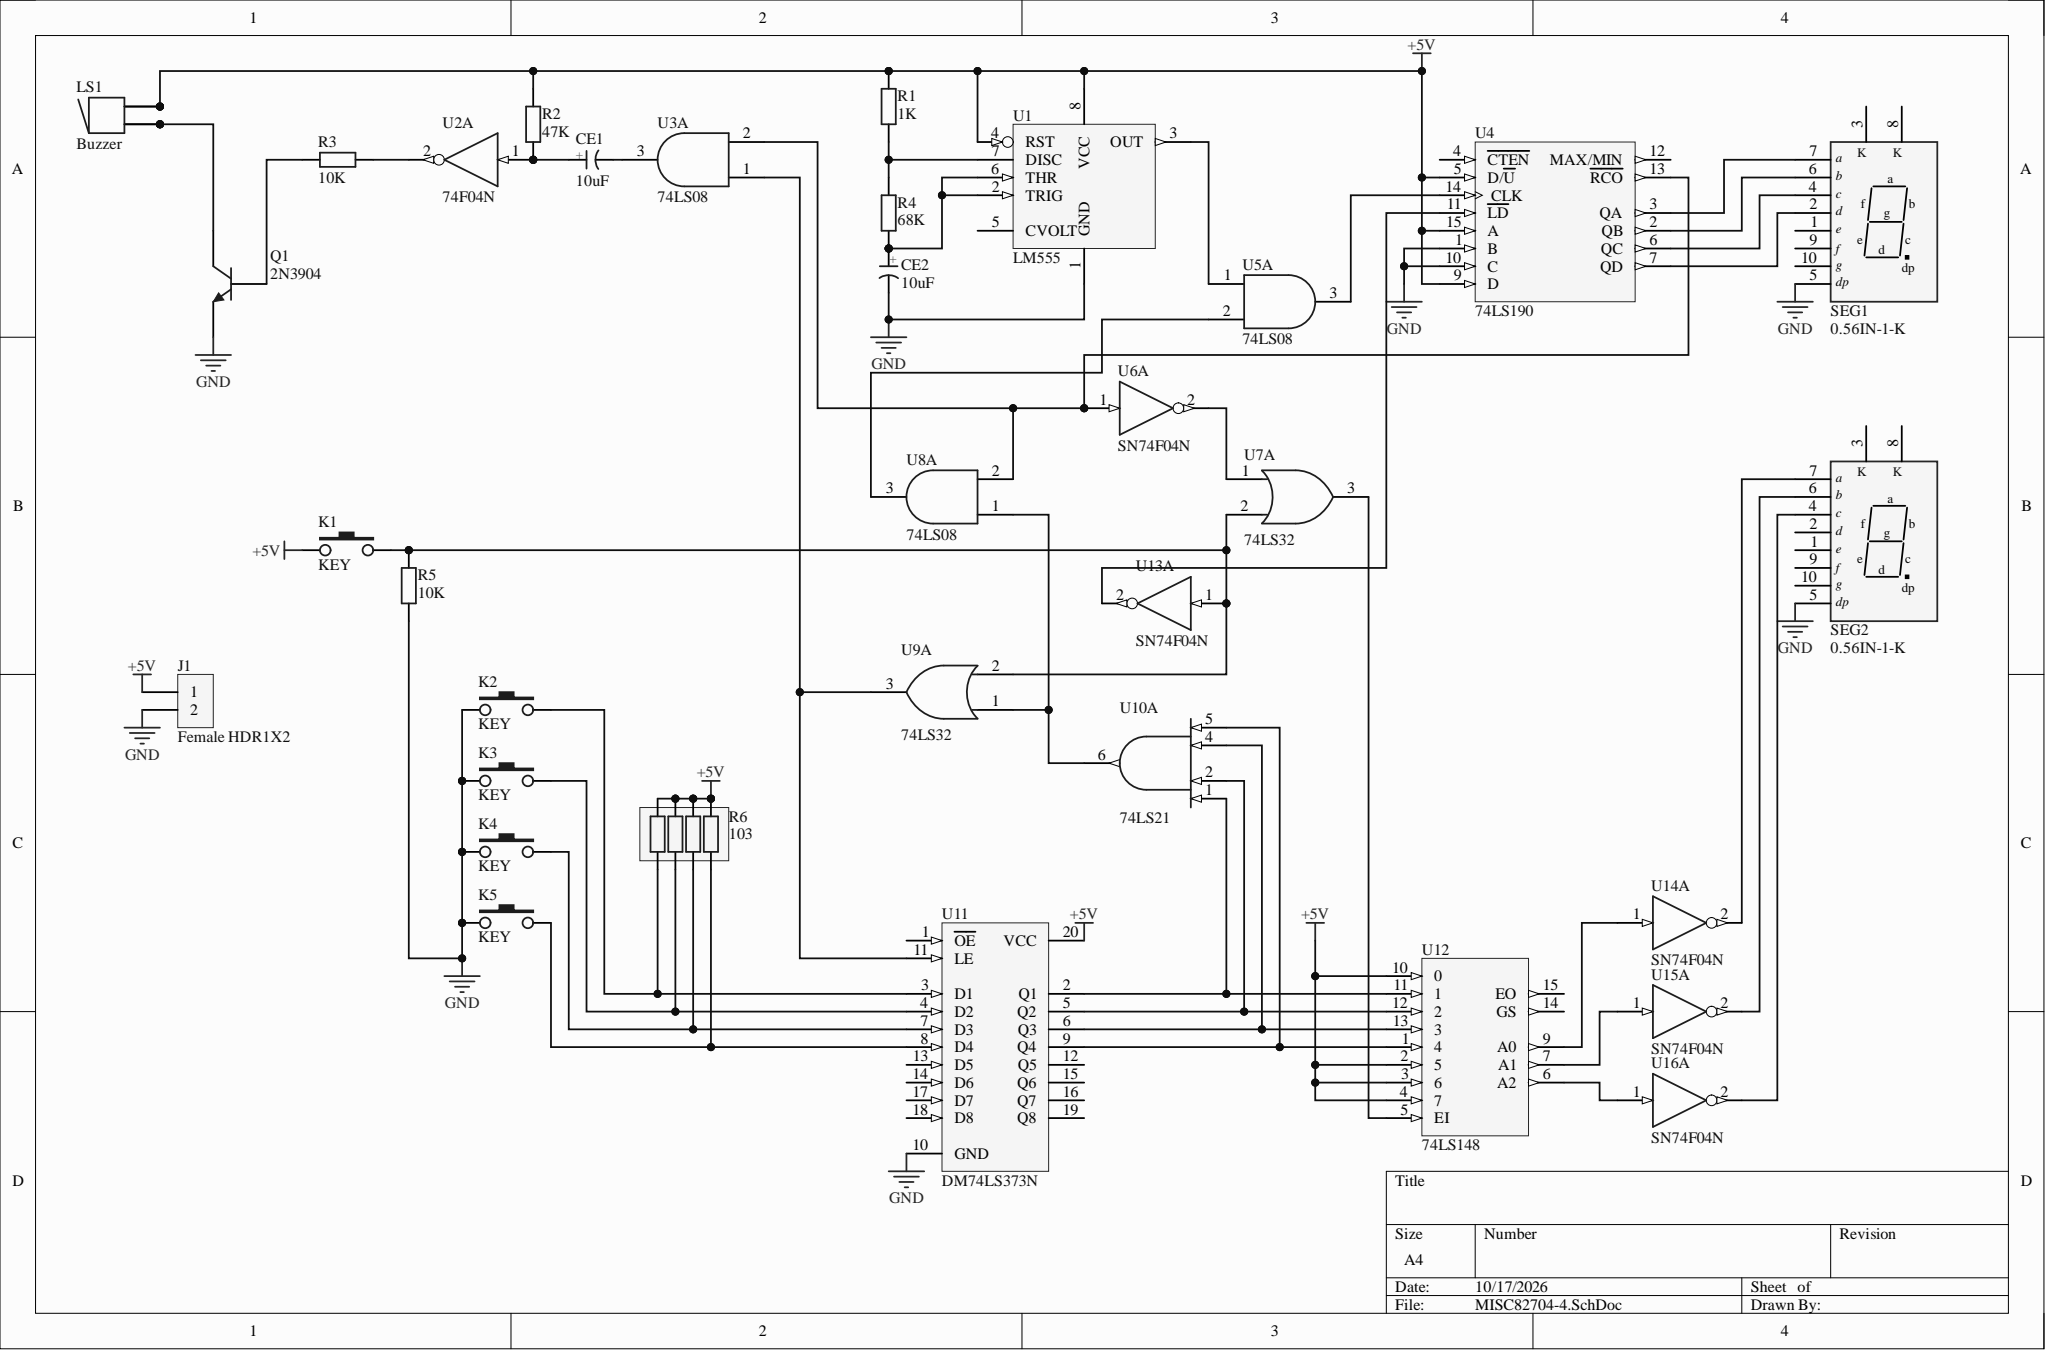Circuit board | Altium Designer | 34 parts | 38 nets
Bill of materials:
Comment,Description,Designator,Footprint,LibRef,Quantity
"10uF","Through-hole electrolytic capacitor","CE1, CE2","CAP 1.5*4*8","CE","2"
"Female HDR1X2","","J1","Fe-HDR1X2/2.54-S","Female HDR1X2","1"
"KEY","","K1, K2, K3, K4, K5","四脚轻触开关","KEY","5"
"Buzzer","Magnetic Transducer Buzzer","LS1","ABSM-1574","Buzzer","1"
"2N3904","NPN General Purpose Amplifier","Q1","TO-92A","2N3904","1"
"1K","Color-band resistor","R1","RS 1/4W","R-S","1"
"47K","Color-band resistor","R2","RS 1/4W","R-S","1"
"10K","Color-band resistor","R3, R5","RS 1/4W","R-S","2"
"68K","Color-band resistor","R4","RS 1/4W","R-S","1"
"103","SMD resistor network","R6","RCA-8P4R-0603","R-8P4R","1"
"0.56IN-1-K","1-digit 0.56-inch common-cathode display","SEG1, SEG2","0.56IN-1P","0.56IN-1-K","2"
"LM555","Timer","U1","J08A","LM555J","1"
"74F04N","Hex Inverter","U2","DIP14","74F04PC","1"
"74LS08","Quad 2-input AND gate","U3, U5, U8","DIP14","74LS08","3"
"74LS190","Synchronous 4-Bit Up/Down Decade Counter with Down/Up Mode Control","U4","DIP16","74LS190","1"
"SN74F04N","Hex Inverter","U6, U13, U14, U15, U16","DIP14","SN74F04N","5"
"74LS32","Quad 2-input OR gate","U7, U9","DIP14","74LS32","2"
"74LS21","Dual 4-Input Positive-AND Gate","U10","DIP14","74LS21","1"
"DM74LS373N","Tri-State Octal D-Type Transparent Latch and Edge-Triggered Flip-Flop","U11","DIP20","DM74LS373N","1"
"74LS148","8-Line to 3-Line Priority Encoder","U12","DIP16","74LS148","1"
Netlist (Protel format):
[
CE1
CAP 1.5*4*8
10uF



]
[
CE2
CAP 1.5*4*8
10uF



]
[
J1
Fe-HDR1X2/2.54-S
Female HDR1X2



]
[
K1
四脚轻触开关
KEY



]
[
K2
四脚轻触开关
KEY



]
[
K3
四脚轻触开关
KEY



]
[
K4
四脚轻触开关
KEY



]
[
K5
四脚轻触开关
KEY



]
[
LS1
ABSM-1574
Buzzer



]
[
Q1
TO-92A
2N3904



]
[
R1
RS 1/4W
1K



]
[
R2
RS 1/4W
47K



]
[
R3
RS 1/4W
10K



]
[
R4
RS 1/4W
68K



]
[
R5
RS 1/4W
10K



]
[
R6
RCA-8P4R-0603
103



]
[
SEG1
0.56IN-1P
0.56IN-1-K



]
[
SEG2
0.56IN-1P
0.56IN-1-K



]
[
U1
J08A
LM555



]
[
U2
DIP14
74F04N



]
[
U3
DIP14
74LS08



]
[
U4
DIP16
74LS190



]
[
U5
DIP14
74LS08



]
[
U6
DIP14
SN74F04N



]
[
U7
DIP14
74LS32



]
[
U8
DIP14
74LS08



]
[
U9
DIP14
74LS32



]
[
U10
DIP14
74LS21



]
[
U11
DIP20
DM74LS373N



]
[
U12
DIP16
74LS148



]
[
U13
DIP14
SN74F04N



]
[
U14
DIP14
SN74F04N



]
[
U15
DIP14
SN74F04N



]
[
U16
DIP14
SN74F04N



]
(
VCC
U2-14
U4-16
U6-14
U10-14
U12-16
U13-14
U14-14
U15-14
U16-14
)
(
NetU12_9
U12-9
U14-1
)
(
NetU12_7
U12-7
U15-1
)
(
NetU12_6
U12-6
U16-1
)
(
NetU10_5
U10-5
U11-9
U12-1
)
(
NetU10_4
U10-4
U11-6
U12-13
)
(
NetU10_2
U10-2
U11-5
U12-12
)
(
NetU10_1
U10-1
U11-2
U12-11
)
(
NetU8_1
U8-1
U9-1
U10-6
)
(
NetU7_3
U7-3
U12-5
)
(
NetU6_2
U6-2
U7-1
)
(
NetU5_2
U5-2
U8-3
)
(
NetU4_14
U4-14
U5-3
)
(
NetU4_11
U4-11
U13-2
)
(
NetU3_2
U3-2
U4-13
U6-1
U8-2
)
(
NetU3_1
U3-1
U9-3
U11-11
)
(
NetU1_3
U1-3
U5-1
)
(
NetSEG2_7
SEG2-7
U14-2
)
(
NetSEG2_6
SEG2-6
U15-2
)
(
NetSEG2_4
SEG2-4
U16-2
)
(
NetSEG1_7
SEG1-7
U4-3
)
(
NetSEG1_6
SEG1-6
U4-2
)
(
NetSEG1_4
SEG1-4
U4-6
)
(
NetSEG1_2
SEG1-2
U4-7
)
(
NetR3_2
R3-2
U2-2
)
(
NetR1_1
R1-1
R4-2
U1-7
)
(
NetQ1_2
Q1-2
R3-1
)
(
NetLS1_1
LS1-1
LS1-1A
Q1-3
)
(
NetK5_3
K5-3
R6-4
U11-8
)
(
NetK4_3
K4-3
R6-3
U11-7
)
(
NetK3_3
K3-3
R6-2
U11-4
)
(
NetK2_3
K2-3
R6-1
U11-3
)
(
NetK1_3
K1-3
R5-2
U7-2
U9-2
U13-1
)
(
NetCE2_1
CE2-1
R4-1
U1-2
U1-6
)
(
NetCE1_2
CE1-2
U3-3
)
(
NetCE1_1
CE1-1
R2-1
U2-1
)
(
GND
CE2-2
J1-2
K2-1
K3-1
K4-1
K5-1
Q1-1
R5-1
SEG1-5
SEG2-5
U1-1
U2-7
U4-1
U4-8
U4-10
U6-7
U10-7
U11-10
U12-8
U13-7
U14-7
U15-7
U16-7
)
(
+5V
J1-1
K1-1
LS1-2
LS1-2A
R1-2
R2-2
R6-5
R6-6
R6-7
R6-8
U1-4
U1-8
U4-5
U4-9
U4-15
U11-20
U12-2
U12-3
U12-4
U12-10
)